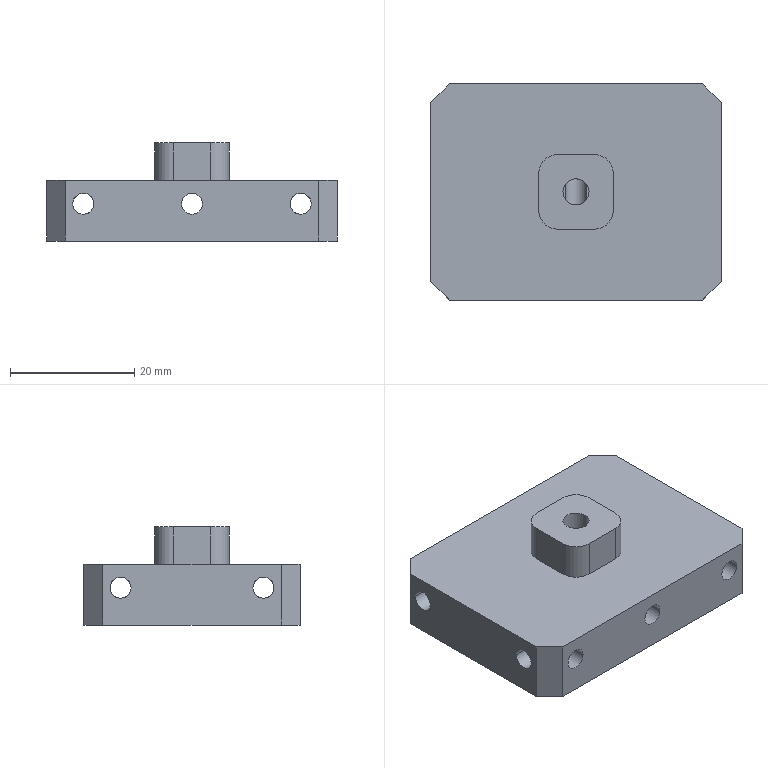Part | STEP file | ASND-0110-TPIM-068 | 1 solid | 66 faces | box 46.8 x 34.8 x 15.8 mm | volume 14684 mm3 | cylinder 49 | plane 17 | commonest cylinder face diameters 3.4 x43 6 x4 4.2 x2